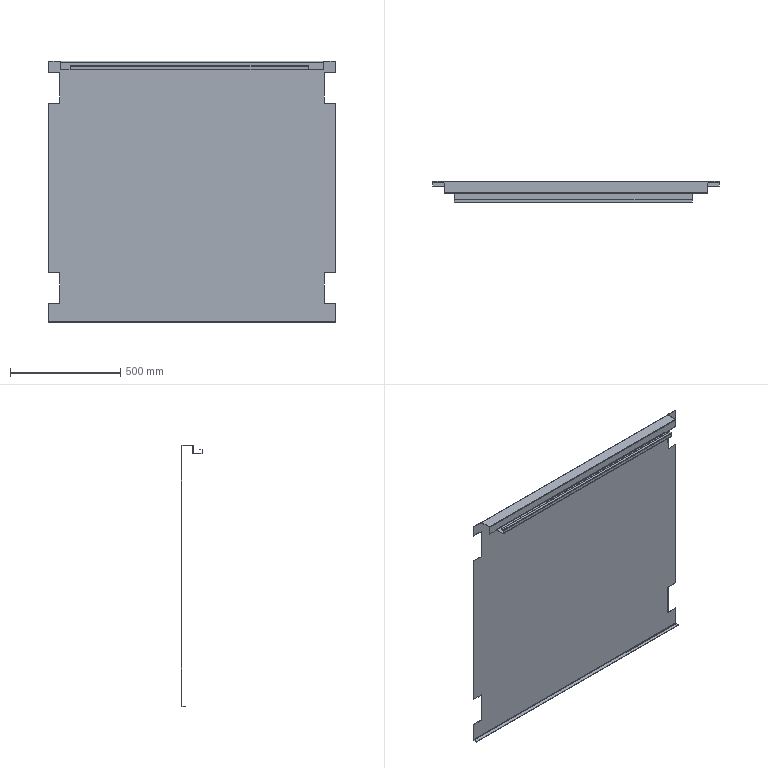Part | SolidWorks | features BaseBody 1 | 1 solid | 86 faces | box 1300 x 97 x 1187 mm | volume 3437938 mm3 | plane 74 | cylinder 12 | commonest cylinder face diameters 2 x6 6 x6